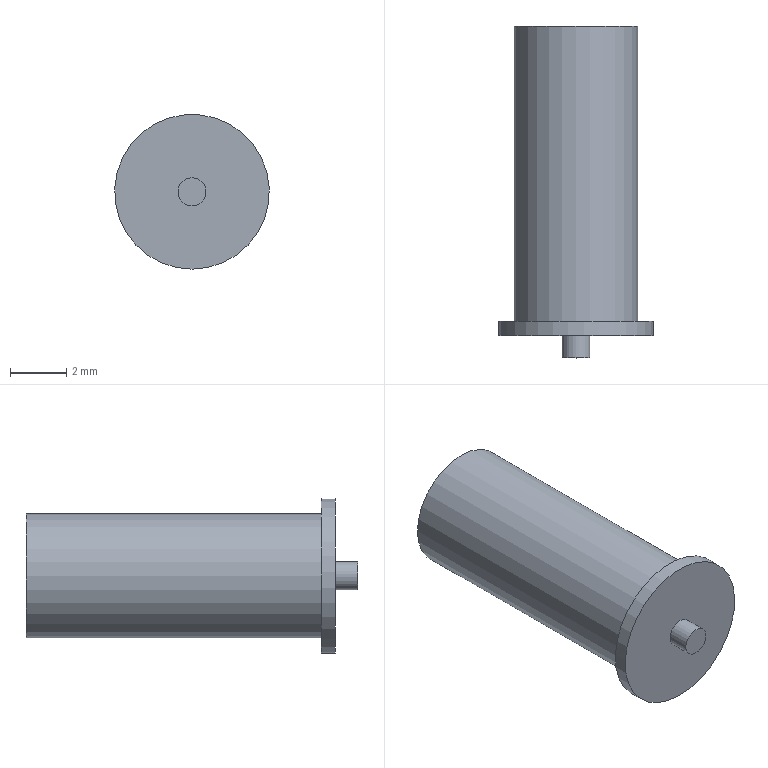Part | STEP file | Copper solder post M3-11-4.4 | 1 solid | 10 faces | box 5.5 x 11.8 x 5.5 mm | volume 131.403 mm3 | cylinder 4 | plane 4 | cone 2 | commonest cylinder face diameters 1 x1 2.5 x1 4.4 x1 5.5 x1
STEP:
#1=CARTESIAN_POINT('',(0.,0.,0.));
#2=DIRECTION('',(0.,0.,1.));
#3=DIRECTION('',(1.,0.,0.));
#4=AXIS2_PLACEMENT_3D('',#1,#2,#3);
#5=CARTESIAN_POINT('',(0.,3.,-1.25));
#6=VERTEX_POINT('',#5);
#7=CARTESIAN_POINT('',(0.,3.,1.25));
#8=VERTEX_POINT('',#7);
#9=CARTESIAN_POINT('',(0.,3.,0.));
#10=DIRECTION('',(0.,1.,0.));
#11=DIRECTION('',(0.,0.,-1.));
#12=AXIS2_PLACEMENT_3D('',#9,#10,#11);
#13=CIRCLE('',#12,1.25);
#14=CARTESIAN_POINT('',(0.,11.,0.));
#15=DIRECTION('',(0.,-1.,0.));
#16=DIRECTION('',(0.,0.,-1.));
#17=AXIS2_PLACEMENT_3D('',#14,#15,#16);
#18=CYLINDRICAL_SURFACE('',#17,1.25);
#19=CARTESIAN_POINT('',(6.283,8.));
#20=DIRECTION('',(-1.,0.));
#21=VECTOR('',#20,1.);
#22=LINE('',#19,#21);
#23=(GEOMETRIC_REPRESENTATION_CONTEXT(2)PARAMETRIC_REPRESENTATION_CONTEXT()REPRESENTATION_CONTEXT('',''));
#24=DEFINITIONAL_REPRESENTATION('',(#22),#23);
#25=PCURVE('',#18,#24);
#26=CARTESIAN_POINT('',(0.,3.,0.));
#27=DIRECTION('',(0.,1.,0.));
#28=DIRECTION('',(0.,0.,1.));
#29=AXIS2_PLACEMENT_3D('',#26,#27,#28);
#30=CONICAL_SURFACE('',#29,1.25,1.03);
#31=CARTESIAN_POINT('',(3.142,0.));
#32=DIRECTION('',(1.,0.));
#33=VECTOR('',#32,1.);
#34=LINE('',#31,#33);
#35=(GEOMETRIC_REPRESENTATION_CONTEXT(2)PARAMETRIC_REPRESENTATION_CONTEXT()REPRESENTATION_CONTEXT('',''));
#36=DEFINITIONAL_REPRESENTATION('',(#34),#35);
#37=PCURVE('',#30,#36);
#38=SURFACE_CURVE('',#13,(#25,#37),.PCURVE_S1.);
#39=EDGE_CURVE('',#6,#8,#38,.T.);
#40=ORIENTED_EDGE('',*,*,#39,.T.);
#41=CARTESIAN_POINT('',(0.,3.,0.));
#42=DIRECTION('',(0.,1.,0.));
#43=DIRECTION('',(0.,0.,-1.));
#44=AXIS2_PLACEMENT_3D('',#41,#42,#43);
#45=CIRCLE('',#44,1.25);
#46=CARTESIAN_POINT('',(6.283,8.));
#47=DIRECTION('',(-1.,0.));
#48=VECTOR('',#47,1.);
#49=LINE('',#46,#48);
#50=(GEOMETRIC_REPRESENTATION_CONTEXT(2)PARAMETRIC_REPRESENTATION_CONTEXT()REPRESENTATION_CONTEXT('',''));
#51=DEFINITIONAL_REPRESENTATION('',(#49),#50);
#52=PCURVE('',#18,#51);
#53=CARTESIAN_POINT('',(-3.142,0.));
#54=DIRECTION('',(1.,0.));
#55=VECTOR('',#54,1.);
#56=LINE('',#53,#55);
#57=(GEOMETRIC_REPRESENTATION_CONTEXT(2)PARAMETRIC_REPRESENTATION_CONTEXT()REPRESENTATION_CONTEXT('',''));
#58=DEFINITIONAL_REPRESENTATION('',(#56),#57);
#59=PCURVE('',#30,#58);
#60=SURFACE_CURVE('',#45,(#52,#59),.PCURVE_S1.);
#61=EDGE_CURVE('',#8,#6,#60,.T.);
#62=ORIENTED_EDGE('',*,*,#61,.T.);
#63=CARTESIAN_POINT('',(0.,10.75,-1.25));
#64=VERTEX_POINT('',#63);
#65=CARTESIAN_POINT('',(0.,10.75,-1.25));
#66=CARTESIAN_POINT('',(0.,3.,-1.25));
#67=B_SPLINE_CURVE_WITH_KNOTS('',1,(#65,#66),.UNSPECIFIED.,.F.,.F.,(2,2),(0.25,8.),.PIECEWISE_BEZIER_KNOTS.);
#68=CARTESIAN_POINT('',(0.,0.));
#69=DIRECTION('',(0.,1.));
#70=VECTOR('',#69,1.);
#71=LINE('',#68,#70);
#72=(GEOMETRIC_REPRESENTATION_CONTEXT(2)PARAMETRIC_REPRESENTATION_CONTEXT()REPRESENTATION_CONTEXT('',''));
#73=DEFINITIONAL_REPRESENTATION('',(#71),#72);
#74=PCURVE('',#18,#73);
#75=CARTESIAN_POINT('',(6.283,0.));
#76=DIRECTION('',(0.,1.));
#77=VECTOR('',#76,1.);
#78=LINE('',#75,#77);
#79=(GEOMETRIC_REPRESENTATION_CONTEXT(2)PARAMETRIC_REPRESENTATION_CONTEXT()REPRESENTATION_CONTEXT('',''));
#80=DEFINITIONAL_REPRESENTATION('',(#78),#79);
#81=PCURVE('',#18,#80);
#82=SEAM_CURVE('',#67,(#74,#81),.PCURVE_S1.);
#83=EDGE_CURVE('',#64,#6,#82,.T.);
#84=ORIENTED_EDGE('',*,*,#83,.F.);
#85=CARTESIAN_POINT('',(0.,10.75,1.25));
#86=VERTEX_POINT('',#85);
#87=CARTESIAN_POINT('',(0.,10.75,0.));
#88=DIRECTION('',(0.,1.,0.));
#89=DIRECTION('',(0.,0.,1.));
#90=AXIS2_PLACEMENT_3D('',#87,#88,#89);
#91=CIRCLE('',#90,1.25);
#92=CARTESIAN_POINT('',(3.142,0.25));
#93=DIRECTION('',(-1.,0.));
#94=VECTOR('',#93,1.);
#95=LINE('',#92,#94);
#96=(GEOMETRIC_REPRESENTATION_CONTEXT(2)PARAMETRIC_REPRESENTATION_CONTEXT()REPRESENTATION_CONTEXT('',''));
#97=DEFINITIONAL_REPRESENTATION('',(#95),#96);
#98=PCURVE('',#18,#97);
#99=CARTESIAN_POINT('',(0.,9.5,0.));
#100=DIRECTION('',(0.,1.,0.));
#101=DIRECTION('',(1.,0.,0.));
#102=AXIS2_PLACEMENT_3D('',#99,#100,#101);
#103=CONICAL_SURFACE('',#102,0.,0.7854);
#104=CARTESIAN_POINT('',(4.712,1.25));
#105=DIRECTION('',(1.,0.));
#106=VECTOR('',#105,1.);
#107=LINE('',#104,#106);
#108=(GEOMETRIC_REPRESENTATION_CONTEXT(2)PARAMETRIC_REPRESENTATION_CONTEXT()REPRESENTATION_CONTEXT('',''));
#109=DEFINITIONAL_REPRESENTATION('',(#107),#108);
#110=PCURVE('',#103,#109);
#111=SURFACE_CURVE('',#91,(#98,#110),.PCURVE_S1.);
#112=EDGE_CURVE('',#86,#64,#111,.T.);
#113=ORIENTED_EDGE('',*,*,#112,.F.);
#114=CARTESIAN_POINT('',(0.,10.75,0.));
#115=DIRECTION('',(0.,1.,0.));
#116=DIRECTION('',(0.,0.,1.));
#117=AXIS2_PLACEMENT_3D('',#114,#115,#116);
#118=CIRCLE('',#117,1.25);
#119=CARTESIAN_POINT('',(9.425,0.25));
#120=DIRECTION('',(-1.,0.));
#121=VECTOR('',#120,1.);
#122=LINE('',#119,#121);
#123=(GEOMETRIC_REPRESENTATION_CONTEXT(2)PARAMETRIC_REPRESENTATION_CONTEXT()REPRESENTATION_CONTEXT('',''));
#124=DEFINITIONAL_REPRESENTATION('',(#122),#123);
#125=PCURVE('',#18,#124);
#126=CARTESIAN_POINT('',(-1.571,1.25));
#127=DIRECTION('',(1.,0.));
#128=VECTOR('',#127,1.);
#129=LINE('',#126,#128);
#130=(GEOMETRIC_REPRESENTATION_CONTEXT(2)PARAMETRIC_REPRESENTATION_CONTEXT()REPRESENTATION_CONTEXT('',''));
#131=DEFINITIONAL_REPRESENTATION('',(#129),#130);
#132=PCURVE('',#103,#131);
#133=SURFACE_CURVE('',#118,(#125,#132),.PCURVE_S1.);
#134=EDGE_CURVE('',#64,#86,#133,.T.);
#135=ORIENTED_EDGE('',*,*,#134,.F.);
#136=ORIENTED_EDGE('',*,*,#83,.T.);
#137=EDGE_LOOP('',(#40,#62,#84,#113,#135,#136));
#138=FACE_BOUND('',#137,.F.);
#139=ADVANCED_FACE('',(#138),#18,.F.);
#140=CARTESIAN_POINT('',(0.,2.249,0.));
#141=VERTEX_POINT('',#140);
#142=CARTESIAN_POINT('',(0.,2.249,0.));
#143=CARTESIAN_POINT('',(0.,3.,1.25));
#144=B_SPLINE_CURVE_WITH_KNOTS('',1,(#142,#143),.UNSPECIFIED.,.F.,.F.,(2,2),(-1.458,0.),.PIECEWISE_BEZIER_KNOTS.);
#145=CARTESIAN_POINT('',(6.283,0.));
#146=DIRECTION('',(0.,1.));
#147=VECTOR('',#146,1.);
#148=LINE('',#145,#147);
#149=(GEOMETRIC_REPRESENTATION_CONTEXT(2)PARAMETRIC_REPRESENTATION_CONTEXT()REPRESENTATION_CONTEXT('',''));
#150=DEFINITIONAL_REPRESENTATION('',(#148),#149);
#151=PCURVE('',#30,#150);
#152=CARTESIAN_POINT('',(0.,0.));
#153=DIRECTION('',(0.,1.));
#154=VECTOR('',#153,1.);
#155=LINE('',#152,#154);
#156=(GEOMETRIC_REPRESENTATION_CONTEXT(2)PARAMETRIC_REPRESENTATION_CONTEXT()REPRESENTATION_CONTEXT('',''));
#157=DEFINITIONAL_REPRESENTATION('',(#155),#156);
#158=PCURVE('',#30,#157);
#159=SEAM_CURVE('',#144,(#151,#158),.PCURVE_S1.);
#160=EDGE_CURVE('',#141,#8,#159,.T.);
#161=ORIENTED_EDGE('',*,*,#160,.T.);
#162=ORIENTED_EDGE('',*,*,#39,.F.);
#163=ORIENTED_EDGE('',*,*,#61,.F.);
#164=ORIENTED_EDGE('',*,*,#160,.F.);
#165=EDGE_LOOP('',(#161,#162,#163,#164));
#166=FACE_BOUND('',#165,.F.);
#167=ADVANCED_FACE('',(#166),#30,.F.);
#168=CARTESIAN_POINT('',(0.,11.,-1.5));
#169=VERTEX_POINT('',#168);
#170=CARTESIAN_POINT('',(0.,11.,0.));
#171=DIRECTION('',(0.,-1.,0.));
#172=DIRECTION('',(0.,0.,-1.));
#173=AXIS2_PLACEMENT_3D('',#170,#171,#172);
#174=CIRCLE('',#173,1.5);
#175=CARTESIAN_POINT('',(7.854,1.5));
#176=DIRECTION('',(-1.,0.));
#177=VECTOR('',#176,1.);
#178=LINE('',#175,#177);
#179=(GEOMETRIC_REPRESENTATION_CONTEXT(2)PARAMETRIC_REPRESENTATION_CONTEXT()REPRESENTATION_CONTEXT('',''));
#180=DEFINITIONAL_REPRESENTATION('',(#178),#179);
#181=PCURVE('',#103,#180);
#182=CARTESIAN_POINT('',(0.,11.,0.));
#183=DIRECTION('',(0.,-1.,0.));
#184=DIRECTION('',(0.,0.,-1.));
#185=AXIS2_PLACEMENT_3D('',#182,#183,#184);
#186=PLANE('',#185);
#187=CARTESIAN_POINT('',(0.,0.));
#188=DIRECTION('',(1.,0.));
#189=AXIS2_PLACEMENT_2D('',#187,#188);
#190=CIRCLE('',#189,1.5);
#191=(GEOMETRIC_REPRESENTATION_CONTEXT(2)PARAMETRIC_REPRESENTATION_CONTEXT()REPRESENTATION_CONTEXT('',''));
#192=DEFINITIONAL_REPRESENTATION('',(#190),#191);
#193=PCURVE('',#186,#192);
#194=SURFACE_CURVE('',#174,(#181,#193),.PCURVE_S1.);
#195=EDGE_CURVE('',#169,#169,#194,.T.);
#196=ORIENTED_EDGE('',*,*,#195,.T.);
#197=CARTESIAN_POINT('',(0.,10.75,-1.25));
#198=CARTESIAN_POINT('',(0.,11.,-1.5));
#199=B_SPLINE_CURVE_WITH_KNOTS('',1,(#197,#198),.UNSPECIFIED.,.F.,.F.,(2,2),(1.768,2.121),.PIECEWISE_BEZIER_KNOTS.);
#200=CARTESIAN_POINT('',(1.571,0.));
#201=DIRECTION('',(0.,1.));
#202=VECTOR('',#201,1.);
#203=LINE('',#200,#202);
#204=(GEOMETRIC_REPRESENTATION_CONTEXT(2)PARAMETRIC_REPRESENTATION_CONTEXT()REPRESENTATION_CONTEXT('',''));
#205=DEFINITIONAL_REPRESENTATION('',(#203),#204);
#206=PCURVE('',#103,#205);
#207=CARTESIAN_POINT('',(7.854,0.));
#208=DIRECTION('',(0.,1.));
#209=VECTOR('',#208,1.);
#210=LINE('',#207,#209);
#211=(GEOMETRIC_REPRESENTATION_CONTEXT(2)PARAMETRIC_REPRESENTATION_CONTEXT()REPRESENTATION_CONTEXT('',''));
#212=DEFINITIONAL_REPRESENTATION('',(#210),#211);
#213=PCURVE('',#103,#212);
#214=SEAM_CURVE('',#199,(#206,#213),.PCURVE_S1.);
#215=EDGE_CURVE('',#64,#169,#214,.T.);
#216=ORIENTED_EDGE('',*,*,#215,.F.);
#217=ORIENTED_EDGE('',*,*,#134,.T.);
#218=ORIENTED_EDGE('',*,*,#112,.T.);
#219=ORIENTED_EDGE('',*,*,#215,.T.);
#220=EDGE_LOOP('',(#196,#216,#217,#218,#219));
#221=FACE_BOUND('',#220,.F.);
#222=ADVANCED_FACE('',(#221),#103,.F.);
#223=CARTESIAN_POINT('',(0.,0.5,-2.2));
#224=VERTEX_POINT('',#223);
#225=CARTESIAN_POINT('',(0.,0.5,0.));
#226=DIRECTION('',(0.,-1.,0.));
#227=DIRECTION('',(0.,0.,-1.));
#228=AXIS2_PLACEMENT_3D('',#225,#226,#227);
#229=CIRCLE('',#228,2.2);
#230=CARTESIAN_POINT('',(-2.2,0.5,0.));
#231=DIRECTION('',(0.,-1.,0.));
#232=DIRECTION('',(0.,0.,-1.));
#233=AXIS2_PLACEMENT_3D('',#230,#231,#232);
#234=PLANE('',#233);
#235=CARTESIAN_POINT('',(0.,2.2));
#236=DIRECTION('',(1.,0.));
#237=AXIS2_PLACEMENT_2D('',#235,#236);
#238=CIRCLE('',#237,2.2);
#239=(GEOMETRIC_REPRESENTATION_CONTEXT(2)PARAMETRIC_REPRESENTATION_CONTEXT()REPRESENTATION_CONTEXT('',''));
#240=DEFINITIONAL_REPRESENTATION('',(#238),#239);
#241=PCURVE('',#234,#240);
#242=CARTESIAN_POINT('',(0.,0.,0.));
#243=DIRECTION('',(0.,-1.,0.));
#244=DIRECTION('',(0.,0.,-1.));
#245=AXIS2_PLACEMENT_3D('',#242,#243,#244);
#246=CYLINDRICAL_SURFACE('',#245,2.2);
#247=CARTESIAN_POINT('',(0.,-0.5));
#248=DIRECTION('',(1.,0.));
#249=VECTOR('',#248,1.);
#250=LINE('',#247,#249);
#251=(GEOMETRIC_REPRESENTATION_CONTEXT(2)PARAMETRIC_REPRESENTATION_CONTEXT()REPRESENTATION_CONTEXT('',''));
#252=DEFINITIONAL_REPRESENTATION('',(#250),#251);
#253=PCURVE('',#246,#252);
#254=SURFACE_CURVE('',#229,(#241,#253),.PCURVE_S1.);
#255=EDGE_CURVE('',#224,#224,#254,.T.);
#256=ORIENTED_EDGE('',*,*,#255,.T.);
#257=EDGE_LOOP('',(#256));
#258=FACE_BOUND('',#257,.T.);
#259=CARTESIAN_POINT('',(0.,0.5,-2.75));
#260=VERTEX_POINT('',#259);
#261=CARTESIAN_POINT('',(0.,0.5,0.));
#262=DIRECTION('',(0.,-1.,0.));
#263=DIRECTION('',(0.,0.,-1.));
#264=AXIS2_PLACEMENT_3D('',#261,#262,#263);
#265=CIRCLE('',#264,2.75);
#266=CARTESIAN_POINT('',(0.,2.2));
#267=DIRECTION('',(1.,0.));
#268=AXIS2_PLACEMENT_2D('',#266,#267);
#269=CIRCLE('',#268,2.75);
#270=(GEOMETRIC_REPRESENTATION_CONTEXT(2)PARAMETRIC_REPRESENTATION_CONTEXT()REPRESENTATION_CONTEXT('',''));
#271=DEFINITIONAL_REPRESENTATION('',(#269),#270);
#272=PCURVE('',#234,#271);
#273=CARTESIAN_POINT('',(0.,0.,0.));
#274=DIRECTION('',(0.,-1.,0.));
#275=DIRECTION('',(0.,0.,-1.));
#276=AXIS2_PLACEMENT_3D('',#273,#274,#275);
#277=CYLINDRICAL_SURFACE('',#276,2.75);
#278=CARTESIAN_POINT('',(0.,-0.5));
#279=DIRECTION('',(1.,0.));
#280=VECTOR('',#279,1.);
#281=LINE('',#278,#280);
#282=(GEOMETRIC_REPRESENTATION_CONTEXT(2)PARAMETRIC_REPRESENTATION_CONTEXT()REPRESENTATION_CONTEXT('',''));
#283=DEFINITIONAL_REPRESENTATION('',(#281),#282);
#284=PCURVE('',#277,#283);
#285=SURFACE_CURVE('',#265,(#272,#284),.PCURVE_S1.);
#286=EDGE_CURVE('',#260,#260,#285,.T.);
#287=ORIENTED_EDGE('',*,*,#286,.F.);
#288=EDGE_LOOP('',(#287));
#289=FACE_BOUND('',#288,.T.);
#290=ADVANCED_FACE('',(#258,#289),#234,.F.);
#291=CARTESIAN_POINT('',(0.,11.,-2.2));
#292=VERTEX_POINT('',#291);
#293=CARTESIAN_POINT('',(0.,11.,0.));
#294=DIRECTION('',(0.,-1.,0.));
#295=DIRECTION('',(0.,0.,-1.));
#296=AXIS2_PLACEMENT_3D('',#293,#294,#295);
#297=CIRCLE('',#296,2.2);
#298=CARTESIAN_POINT('',(0.,-11.));
#299=DIRECTION('',(1.,0.));
#300=VECTOR('',#299,1.);
#301=LINE('',#298,#300);
#302=(GEOMETRIC_REPRESENTATION_CONTEXT(2)PARAMETRIC_REPRESENTATION_CONTEXT()REPRESENTATION_CONTEXT('',''));
#303=DEFINITIONAL_REPRESENTATION('',(#301),#302);
#304=PCURVE('',#246,#303);
#305=CARTESIAN_POINT('',(0.,0.));
#306=DIRECTION('',(1.,0.));
#307=AXIS2_PLACEMENT_2D('',#305,#306);
#308=CIRCLE('',#307,2.2);
#309=(GEOMETRIC_REPRESENTATION_CONTEXT(2)PARAMETRIC_REPRESENTATION_CONTEXT()REPRESENTATION_CONTEXT('',''));
#310=DEFINITIONAL_REPRESENTATION('',(#308),#309);
#311=PCURVE('',#186,#310);
#312=SURFACE_CURVE('',#297,(#304,#311),.PCURVE_S1.);
#313=EDGE_CURVE('',#292,#292,#312,.T.);
#314=ORIENTED_EDGE('',*,*,#313,.T.);
#315=CARTESIAN_POINT('',(0.,11.,-2.2));
#316=CARTESIAN_POINT('',(0.,0.5,-2.2));
#317=B_SPLINE_CURVE_WITH_KNOTS('',1,(#315,#316),.UNSPECIFIED.,.F.,.F.,(2,2),(-11.,-0.5),.PIECEWISE_BEZIER_KNOTS.);
#318=CARTESIAN_POINT('',(6.283,0.));
#319=DIRECTION('',(0.,1.));
#320=VECTOR('',#319,1.);
#321=LINE('',#318,#320);
#322=(GEOMETRIC_REPRESENTATION_CONTEXT(2)PARAMETRIC_REPRESENTATION_CONTEXT()REPRESENTATION_CONTEXT('',''));
#323=DEFINITIONAL_REPRESENTATION('',(#321),#322);
#324=PCURVE('',#246,#323);
#325=CARTESIAN_POINT('',(0.,0.));
#326=DIRECTION('',(0.,1.));
#327=VECTOR('',#326,1.);
#328=LINE('',#325,#327);
#329=(GEOMETRIC_REPRESENTATION_CONTEXT(2)PARAMETRIC_REPRESENTATION_CONTEXT()REPRESENTATION_CONTEXT('',''));
#330=DEFINITIONAL_REPRESENTATION('',(#328),#329);
#331=PCURVE('',#246,#330);
#332=SEAM_CURVE('',#317,(#324,#331),.PCURVE_S1.);
#333=EDGE_CURVE('',#292,#224,#332,.T.);
#334=ORIENTED_EDGE('',*,*,#333,.T.);
#335=ORIENTED_EDGE('',*,*,#255,.F.);
#336=ORIENTED_EDGE('',*,*,#333,.F.);
#337=EDGE_LOOP('',(#314,#334,#335,#336));
#338=FACE_BOUND('',#337,.T.);
#339=ADVANCED_FACE('',(#338),#246,.T.);
#340=ORIENTED_EDGE('',*,*,#313,.F.);
#341=EDGE_LOOP('',(#340));
#342=FACE_BOUND('',#341,.T.);
#343=ORIENTED_EDGE('',*,*,#195,.T.);
#344=EDGE_LOOP('',(#343));
#345=FACE_BOUND('',#344,.T.);
#346=ADVANCED_FACE('',(#342,#345),#186,.F.);
#347=CARTESIAN_POINT('',(0.,-0.8,-0.5));
#348=VERTEX_POINT('',#347);
#349=CARTESIAN_POINT('',(0.,-0.8,0.));
#350=DIRECTION('',(0.,-1.,0.));
#351=DIRECTION('',(0.,0.,-1.));
#352=AXIS2_PLACEMENT_3D('',#349,#350,#351);
#353=CIRCLE('',#352,0.5);
#354=CARTESIAN_POINT('',(-0.5,-0.8,0.));
#355=DIRECTION('',(0.,1.,0.));
#356=DIRECTION('',(0.,0.,1.));
#357=AXIS2_PLACEMENT_3D('',#354,#355,#356);
#358=PLANE('',#357);
#359=CARTESIAN_POINT('',(-0.5,0.5));
#360=CARTESIAN_POINT('',(-0.5,1.366));
#361=CARTESIAN_POINT('',(0.25,0.933));
#362=CARTESIAN_POINT('',(1.,0.5));
#363=CARTESIAN_POINT('',(0.25,0.06699));
#364=CARTESIAN_POINT('',(-0.5,-0.366));
#365=CARTESIAN_POINT('',(-0.5,0.5));
#366=(BOUNDED_CURVE()B_SPLINE_CURVE(2,(#359,#360,#361,#362,#363,#364,#365),.UNSPECIFIED.,.T.,.F.)B_SPLINE_CURVE_WITH_KNOTS((1,2,2,2,2,1),(-2.094,0.,2.094,4.189,6.283,8.378),.UNSPECIFIED.)CURVE()GEOMETRIC_REPRESENTATION_ITEM()RATIONAL_B_SPLINE_CURVE((1.,0.5,1.,0.5,1.,0.5,1.))REPRESENTATION_ITEM(''));
#367=(GEOMETRIC_REPRESENTATION_CONTEXT(2)PARAMETRIC_REPRESENTATION_CONTEXT()REPRESENTATION_CONTEXT('',''));
#368=DEFINITIONAL_REPRESENTATION('',(#366),#367);
#369=PCURVE('',#358,#368);
#370=CARTESIAN_POINT('',(0.,0.,0.));
#371=DIRECTION('',(0.,-1.,0.));
#372=DIRECTION('',(0.,0.,-1.));
#373=AXIS2_PLACEMENT_3D('',#370,#371,#372);
#374=CYLINDRICAL_SURFACE('',#373,0.5);
#375=CARTESIAN_POINT('',(0.,0.8));
#376=DIRECTION('',(1.,0.));
#377=VECTOR('',#376,1.);
#378=LINE('',#375,#377);
#379=(GEOMETRIC_REPRESENTATION_CONTEXT(2)PARAMETRIC_REPRESENTATION_CONTEXT()REPRESENTATION_CONTEXT('',''));
#380=DEFINITIONAL_REPRESENTATION('',(#378),#379);
#381=PCURVE('',#374,#380);
#382=SURFACE_CURVE('',#353,(#369,#381),.PCURVE_S1.);
#383=EDGE_CURVE('',#348,#348,#382,.T.);
#384=ORIENTED_EDGE('',*,*,#383,.T.);
#385=EDGE_LOOP('',(#384));
#386=FACE_BOUND('',#385,.T.);
#387=ADVANCED_FACE('',(#386),#358,.F.);
#388=CARTESIAN_POINT('',(0.,0.,-0.5));
#389=VERTEX_POINT('',#388);
#390=CARTESIAN_POINT('',(0.,0.,0.));
#391=DIRECTION('',(0.,-1.,0.));
#392=DIRECTION('',(0.,0.,-1.));
#393=AXIS2_PLACEMENT_3D('',#390,#391,#392);
#394=CIRCLE('',#393,0.5);
#395=CARTESIAN_POINT('',(0.,0.));
#396=DIRECTION('',(1.,0.));
#397=VECTOR('',#396,1.);
#398=LINE('',#395,#397);
#399=(GEOMETRIC_REPRESENTATION_CONTEXT(2)PARAMETRIC_REPRESENTATION_CONTEXT()REPRESENTATION_CONTEXT('',''));
#400=DEFINITIONAL_REPRESENTATION('',(#398),#399);
#401=PCURVE('',#374,#400);
#402=CARTESIAN_POINT('',(-2.75,0.,0.));
#403=DIRECTION('',(0.,1.,0.));
#404=DIRECTION('',(0.,0.,1.));
#405=AXIS2_PLACEMENT_3D('',#402,#403,#404);
#406=PLANE('',#405);
#407=CARTESIAN_POINT('',(-0.5,2.75));
#408=CARTESIAN_POINT('',(-0.5,3.616));
#409=CARTESIAN_POINT('',(0.25,3.183));
#410=CARTESIAN_POINT('',(1.,2.75));
#411=CARTESIAN_POINT('',(0.25,2.317));
#412=CARTESIAN_POINT('',(-0.5,1.884));
#413=CARTESIAN_POINT('',(-0.5,2.75));
#414=(BOUNDED_CURVE()B_SPLINE_CURVE(2,(#407,#408,#409,#410,#411,#412,#413),.UNSPECIFIED.,.T.,.F.)B_SPLINE_CURVE_WITH_KNOTS((1,2,2,2,2,1),(-2.094,0.,2.094,4.189,6.283,8.378),.UNSPECIFIED.)CURVE()GEOMETRIC_REPRESENTATION_ITEM()RATIONAL_B_SPLINE_CURVE((1.,0.5,1.,0.5,1.,0.5,1.))REPRESENTATION_ITEM(''));
#415=(GEOMETRIC_REPRESENTATION_CONTEXT(2)PARAMETRIC_REPRESENTATION_CONTEXT()REPRESENTATION_CONTEXT('',''));
#416=DEFINITIONAL_REPRESENTATION('',(#414),#415);
#417=PCURVE('',#406,#416);
#418=SURFACE_CURVE('',#394,(#401,#417),.PCURVE_S1.);
#419=EDGE_CURVE('',#389,#389,#418,.T.);
#420=ORIENTED_EDGE('',*,*,#419,.T.);
#421=CARTESIAN_POINT('',(0.,0.,-0.5));
#422=CARTESIAN_POINT('',(0.,-0.8,-0.5));
#423=B_SPLINE_CURVE_WITH_KNOTS('',1,(#421,#422),.UNSPECIFIED.,.F.,.F.,(2,2),(0.,0.8),.PIECEWISE_BEZIER_KNOTS.);
#424=CARTESIAN_POINT('',(6.283,0.));
#425=DIRECTION('',(0.,1.));
#426=VECTOR('',#425,1.);
#427=LINE('',#424,#426);
#428=(GEOMETRIC_REPRESENTATION_CONTEXT(2)PARAMETRIC_REPRESENTATION_CONTEXT()REPRESENTATION_CONTEXT('',''));
#429=DEFINITIONAL_REPRESENTATION('',(#427),#428);
#430=PCURVE('',#374,#429);
#431=CARTESIAN_POINT('',(0.,0.));
#432=DIRECTION('',(0.,1.));
#433=VECTOR('',#432,1.);
#434=LINE('',#431,#433);
#435=(GEOMETRIC_REPRESENTATION_CONTEXT(2)PARAMETRIC_REPRESENTATION_CONTEXT()REPRESENTATION_CONTEXT('',''));
#436=DEFINITIONAL_REPRESENTATION('',(#434),#435);
#437=PCURVE('',#374,#436);
#438=SEAM_CURVE('',#423,(#430,#437),.PCURVE_S1.);
#439=EDGE_CURVE('',#389,#348,#438,.T.);
#440=ORIENTED_EDGE('',*,*,#439,.T.);
#441=ORIENTED_EDGE('',*,*,#383,.F.);
#442=ORIENTED_EDGE('',*,*,#439,.F.);
#443=EDGE_LOOP('',(#420,#440,#441,#442));
#444=FACE_BOUND('',#443,.T.);
#445=ADVANCED_FACE('',(#444),#374,.T.);
#446=CARTESIAN_POINT('',(0.,0.,-2.75));
#447=VERTEX_POINT('',#446);
#448=CARTESIAN_POINT('',(0.,0.,0.));
#449=DIRECTION('',(0.,-1.,0.));
#450=DIRECTION('',(0.,0.,-1.));
#451=AXIS2_PLACEMENT_3D('',#448,#449,#450);
#452=CIRCLE('',#451,2.75);
#453=CARTESIAN_POINT('',(-2.75,2.75));
#454=CARTESIAN_POINT('',(-2.75,7.513));
#455=CARTESIAN_POINT('',(1.375,5.132));
#456=CARTESIAN_POINT('',(5.5,2.75));
#457=CARTESIAN_POINT('',(1.375,0.3684));
#458=CARTESIAN_POINT('',(-2.75,-2.013));
#459=CARTESIAN_POINT('',(-2.75,2.75));
#460=(BOUNDED_CURVE()B_SPLINE_CURVE(2,(#453,#454,#455,#456,#457,#458,#459),.UNSPECIFIED.,.T.,.F.)B_SPLINE_CURVE_WITH_KNOTS((1,2,2,2,2,1),(-2.094,0.,2.094,4.189,6.283,8.378),.UNSPECIFIED.)CURVE()GEOMETRIC_REPRESENTATION_ITEM()RATIONAL_B_SPLINE_CURVE((1.,0.5,1.,0.5,1.,0.5,1.))REPRESENTATION_ITEM(''));
#461=(GEOMETRIC_REPRESENTATION_CONTEXT(2)PARAMETRIC_REPRESENTATION_CONTEXT()REPRESENTATION_CONTEXT('',''));
#462=DEFINITIONAL_REPRESENTATION('',(#460),#461);
#463=PCURVE('',#406,#462);
#464=CARTESIAN_POINT('',(0.,0.));
#465=DIRECTION('',(1.,0.));
#466=VECTOR('',#465,1.);
#467=LINE('',#464,#466);
#468=(GEOMETRIC_REPRESENTATION_CONTEXT(2)PARAMETRIC_REPRESENTATION_CONTEXT()REPRESENTATION_CONTEXT('',''));
#469=DEFINITIONAL_REPRESENTATION('',(#467),#468);
#470=PCURVE('',#277,#469);
#471=SURFACE_CURVE('',#452,(#463,#470),.PCURVE_S1.);
#472=EDGE_CURVE('',#447,#447,#471,.T.);
#473=ORIENTED_EDGE('',*,*,#472,.T.);
#474=EDGE_LOOP('',(#473));
#475=FACE_BOUND('',#474,.T.);
#476=ORIENTED_EDGE('',*,*,#419,.F.);
#477=EDGE_LOOP('',(#476));
#478=FACE_BOUND('',#477,.T.);
#479=ADVANCED_FACE('',(#475,#478),#406,.F.);
#480=ORIENTED_EDGE('',*,*,#286,.T.);
#481=CARTESIAN_POINT('',(0.,0.5,-2.75));
#482=CARTESIAN_POINT('',(0.,0.,-2.75));
#483=B_SPLINE_CURVE_WITH_KNOTS('',1,(#481,#482),.UNSPECIFIED.,.F.,.F.,(2,2),(-0.5,0.),.PIECEWISE_BEZIER_KNOTS.);
#484=CARTESIAN_POINT('',(6.283,0.));
#485=DIRECTION('',(0.,1.));
#486=VECTOR('',#485,1.);
#487=LINE('',#484,#486);
#488=(GEOMETRIC_REPRESENTATION_CONTEXT(2)PARAMETRIC_REPRESENTATION_CONTEXT()REPRESENTATION_CONTEXT('',''));
#489=DEFINITIONAL_REPRESENTATION('',(#487),#488);
#490=PCURVE('',#277,#489);
#491=CARTESIAN_POINT('',(0.,0.));
#492=DIRECTION('',(0.,1.));
#493=VECTOR('',#492,1.);
#494=LINE('',#491,#493);
#495=(GEOMETRIC_REPRESENTATION_CONTEXT(2)PARAMETRIC_REPRESENTATION_CONTEXT()REPRESENTATION_CONTEXT('',''));
#496=DEFINITIONAL_REPRESENTATION('',(#494),#495);
#497=PCURVE('',#277,#496);
#498=SEAM_CURVE('',#483,(#490,#497),.PCURVE_S1.);
#499=EDGE_CURVE('',#260,#447,#498,.T.);
#500=ORIENTED_EDGE('',*,*,#499,.T.);
#501=ORIENTED_EDGE('',*,*,#472,.F.);
#502=ORIENTED_EDGE('',*,*,#499,.F.);
#503=EDGE_LOOP('',(#480,#500,#501,#502));
#504=FACE_BOUND('',#503,.T.);
#505=ADVANCED_FACE('',(#504),#277,.T.);
#506=CLOSED_SHELL('',(#139,#167,#222,#290,#339,#346,#387,#445,#479,#505));
#507=MANIFOLD_SOLID_BREP('',#506);
#508=(LENGTH_UNIT()NAMED_UNIT(*)SI_UNIT(.MILLI.,.METRE.));
#509=UNCERTAINTY_MEASURE_WITH_UNIT(LENGTH_MEASURE(0.00001),#508,'','');
#510=(NAMED_UNIT(*)PLANE_ANGLE_UNIT()SI_UNIT($,.RADIAN.));
#511=(NAMED_UNIT(*)SI_UNIT($,.STERADIAN.)SOLID_ANGLE_UNIT());
#512=(GEOMETRIC_REPRESENTATION_CONTEXT(3)GLOBAL_UNCERTAINTY_ASSIGNED_CONTEXT((#509))GLOBAL_UNIT_ASSIGNED_CONTEXT((#508,#510,#511))REPRESENTATION_CONTEXT('',''));
#513=ADVANCED_BREP_SHAPE_REPRESENTATION('',(#4,#507),#512);